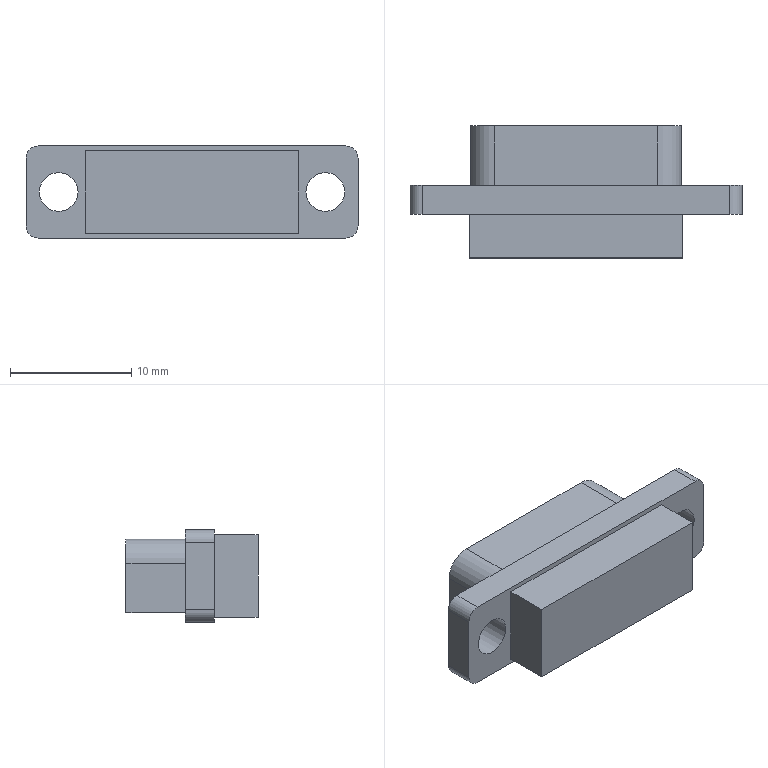Part | STEP file | J30J-21TK | 1 solid | 31 faces | box 27.4 x 10.9 x 7.6 mm | volume 1017 mm3 | plane 21 | cylinder 10 | commonest cylinder face diameters 2 x4 1 x2 3.2 x2 4 x2